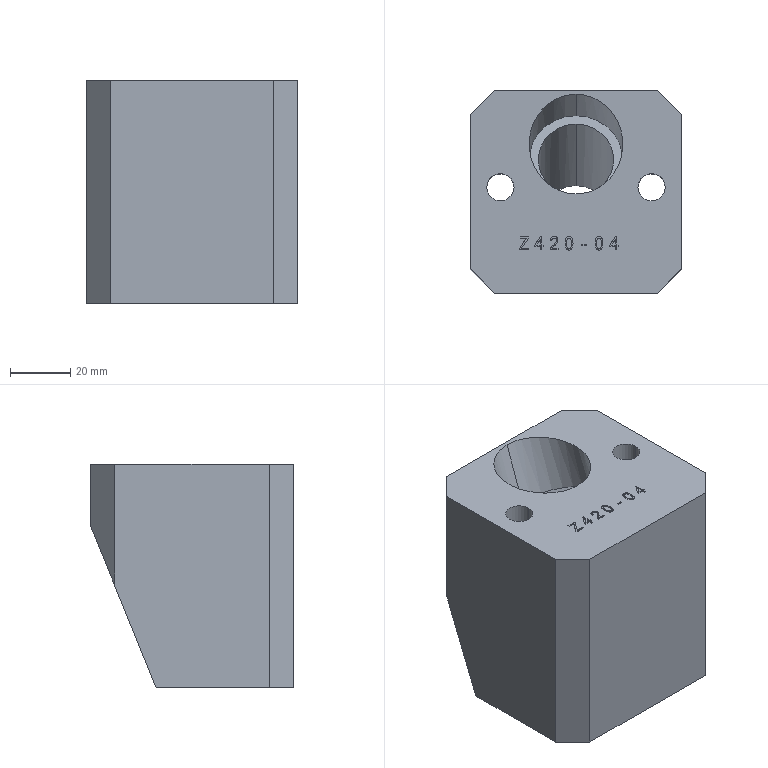Part | Creo | 1 solid | 143 faces | box 70 x 67 x 74 mm | volume 246330 mm3 | other 65 | plane 64 | cylinder 14 | commonest cylinder face diameters 9 x4 15 x4 25 x2 31 x2 3.854 x1 60.776 x1